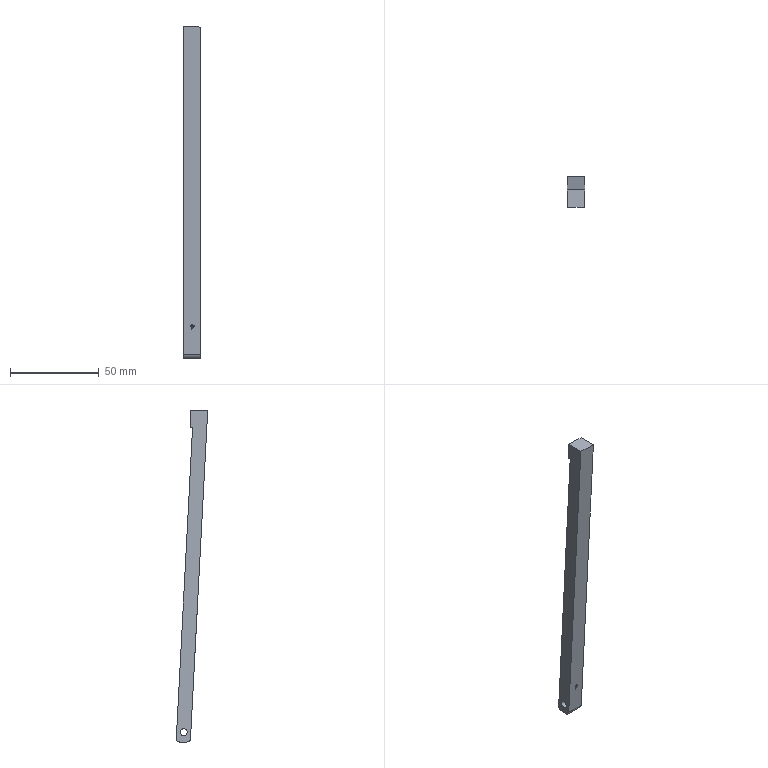Part | STEP file | solid 25 | 1 solid | 42 faces | box 10 x 17.713 x 187.185 mm | volume 14965 mm3 | plane 37 | cylinder 5 | commonest cylinder face diameters 4 x3 1.005 x1 6922 x1